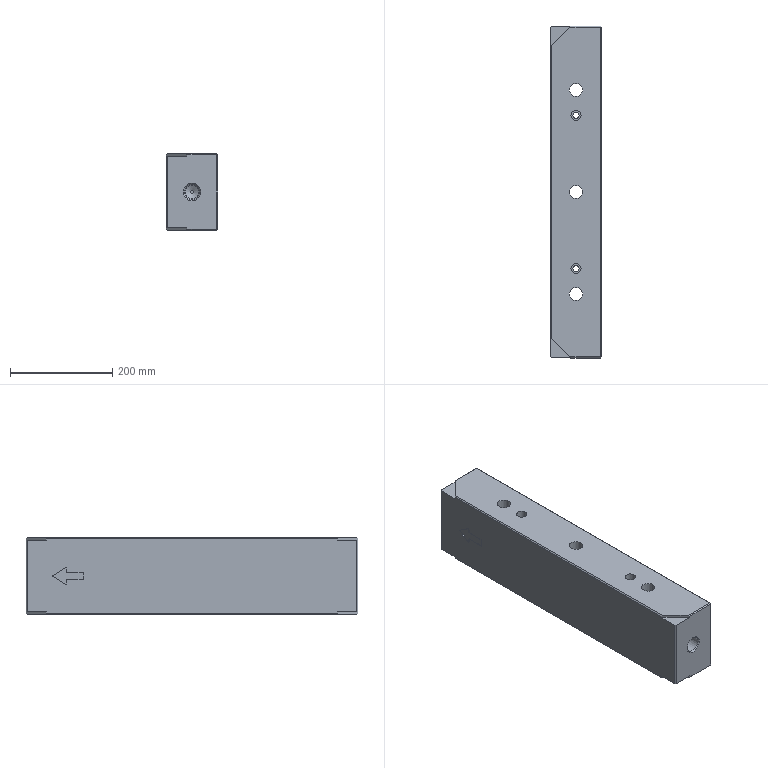Part | STEP file | P011002C002-000 | 1 solid | 110 faces | box 100 x 650 x 150 mm | volume 9316840 mm3 | plane 60 | cylinder 32 | cone 18 | commonest cylinder face diameters 1.5 x7 14 x4 15.947 x4 16 x4 20 x4 26 x3